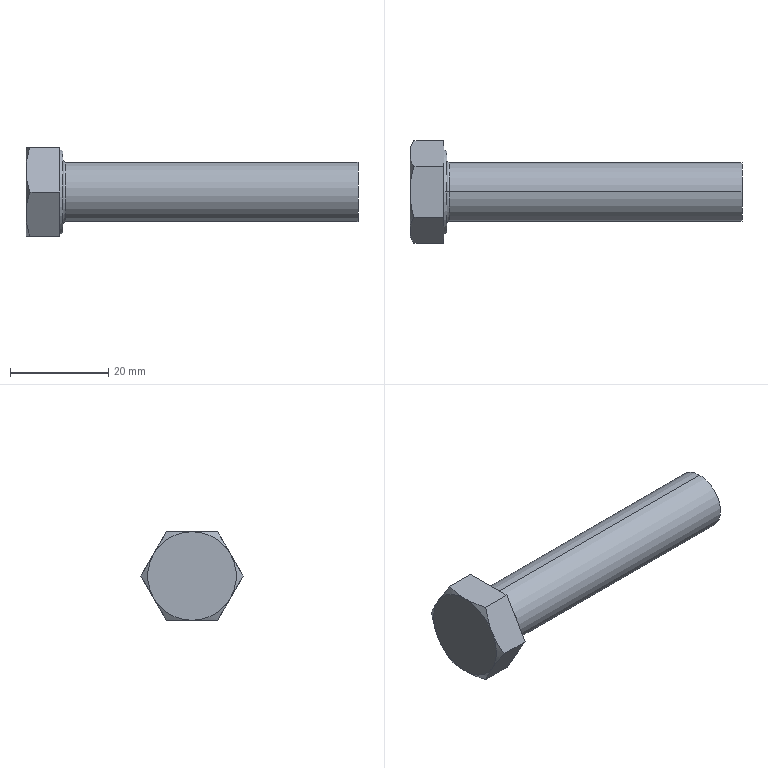Part | SolidWorks | features RevCut 3, Extrusion 1, Fillet 1, LPattern 1, Revolution 1 | 1 solid | 22 faces | box 67.5 x 20.785 x 18 mm | volume 8854 mm3 | plane 10 | cone 8 | torus 2 | cylinder 2 | commonest cylinder face diameters 12 x2
STEP:
#1=CARTESIAN_POINT('',(8.1,0.,6.));
#2=VERTEX_POINT('',#1);
#3=CARTESIAN_POINT('',(8.1,0.,-6.));
#4=VERTEX_POINT('',#3);
#5=CARTESIAN_POINT('',(8.1,0.,0.));
#6=DIRECTION('',(1.,0.,0.));
#7=DIRECTION('',(0.,0.,-1.));
#8=AXIS2_PLACEMENT_3D('',#5,#6,#7);
#9=CIRCLE('',#8,6.);
#10=EDGE_CURVE('',#2,#4,#9,.T.);
#11=ORIENTED_EDGE('',*,*,#10,.F.);
#12=CARTESIAN_POINT('',(7.5,0.,6.6));
#13=VERTEX_POINT('',#12);
#14=CARTESIAN_POINT('',(8.1,0.,6.6));
#15=DIRECTION('',(0.,1.,0.));
#16=DIRECTION('',(0.,0.,1.));
#17=AXIS2_PLACEMENT_3D('',#14,#15,#16);
#18=CIRCLE('',#17,0.6);
#19=EDGE_CURVE('',#2,#13,#18,.T.);
#20=ORIENTED_EDGE('',*,*,#19,.T.);
#21=CARTESIAN_POINT('',(7.5,0.,-6.6));
#22=VERTEX_POINT('',#21);
#23=CARTESIAN_POINT('',(7.5,0.,0.));
#24=DIRECTION('',(-1.,0.,0.));
#25=DIRECTION('',(0.,0.,-1.));
#26=AXIS2_PLACEMENT_3D('',#23,#24,#25);
#27=CIRCLE('',#26,6.6);
#28=EDGE_CURVE('',#22,#13,#27,.T.);
#29=ORIENTED_EDGE('',*,*,#28,.F.);
#30=CARTESIAN_POINT('',(8.1,0.,-6.6));
#31=DIRECTION('',(0.,-1.,0.));
#32=DIRECTION('',(0.,0.,-1.));
#33=AXIS2_PLACEMENT_3D('',#30,#31,#32);
#34=CIRCLE('',#33,0.6);
#35=EDGE_CURVE('',#4,#22,#34,.T.);
#36=ORIENTED_EDGE('',*,*,#35,.F.);
#37=EDGE_LOOP('',(#11,#20,#29,#36));
#38=FACE_OUTER_BOUND('',#37,.T.);
#39=CARTESIAN_POINT('',(8.1,0.,0.));
#40=DIRECTION('',(1.,0.,0.));
#41=DIRECTION('',(0.,0.,-1.));
#42=AXIS2_PLACEMENT_3D('',#39,#40,#41);
#43=TOROIDAL_SURFACE('',#42,6.6,0.6);
#44=ADVANCED_FACE('',(#38),#43,.F.);
#45=CARTESIAN_POINT('',(67.5,0.,6.));
#46=VERTEX_POINT('',#45);
#47=CARTESIAN_POINT('',(67.5,0.,-6.));
#48=VERTEX_POINT('',#47);
#49=CARTESIAN_POINT('',(67.5,0.,0.));
#50=DIRECTION('',(-1.,0.,0.));
#51=DIRECTION('',(0.,0.,1.));
#52=AXIS2_PLACEMENT_3D('',#49,#50,#51);
#53=CIRCLE('',#52,6.);
#54=EDGE_CURVE('',#46,#48,#53,.T.);
#55=ORIENTED_EDGE('',*,*,#54,.T.);
#56=CARTESIAN_POINT('',(0.,0.,-6.));
#57=DIRECTION('',(-1.,0.,0.));
#58=VECTOR('',#57,1000.);
#59=LINE('',#56,#58);
#60=EDGE_CURVE('',#48,#4,#59,.T.);
#61=ORIENTED_EDGE('',*,*,#60,.T.);
#62=CARTESIAN_POINT('',(8.1,0.,0.));
#63=DIRECTION('',(1.,0.,0.));
#64=DIRECTION('',(0.,0.,-1.));
#65=AXIS2_PLACEMENT_3D('',#62,#63,#64);
#66=CIRCLE('',#65,6.);
#67=EDGE_CURVE('',#4,#2,#66,.T.);
#68=ORIENTED_EDGE('',*,*,#67,.T.);
#69=CARTESIAN_POINT('',(0.,0.,6.));
#70=DIRECTION('',(-1.,0.,0.));
#71=VECTOR('',#70,1000.);
#72=LINE('',#69,#71);
#73=EDGE_CURVE('',#46,#2,#72,.T.);
#74=ORIENTED_EDGE('',*,*,#73,.F.);
#75=EDGE_LOOP('',(#55,#61,#68,#74));
#76=FACE_OUTER_BOUND('',#75,.T.);
#77=CARTESIAN_POINT('',(0.,0.,0.));
#78=DIRECTION('',(-1.,0.,0.));
#79=DIRECTION('',(0.,0.,1.));
#80=AXIS2_PLACEMENT_3D('',#77,#78,#79);
#81=CYLINDRICAL_SURFACE('',#80,6.);
#82=ADVANCED_FACE('',(#76),#81,.T.);
#83=CARTESIAN_POINT('',(7.5,0.,8.315));
#84=VERTEX_POINT('',#83);
#85=CARTESIAN_POINT('',(7.5,0.,-8.315));
#86=VERTEX_POINT('',#85);
#87=CARTESIAN_POINT('',(7.5,0.,0.));
#88=DIRECTION('',(-1.,0.,0.));
#89=DIRECTION('',(0.,0.,1.));
#90=AXIS2_PLACEMENT_3D('',#87,#88,#89);
#91=CIRCLE('',#90,8.315);
#92=EDGE_CURVE('',#84,#86,#91,.T.);
#93=ORIENTED_EDGE('',*,*,#92,.T.);
#94=CARTESIAN_POINT('',(6.9,0.,-8.661));
#95=VERTEX_POINT('',#94);
#96=CARTESIAN_POINT('',(6.9,0.,-8.661));
#97=DIRECTION('',(-0.866,0.,-0.5));
#98=VECTOR('',#97,1000.);
#99=LINE('',#96,#98);
#100=EDGE_CURVE('',#86,#95,#99,.T.);
#101=ORIENTED_EDGE('',*,*,#100,.T.);
#102=CARTESIAN_POINT('',(6.9,0.,8.661));
#103=VERTEX_POINT('',#102);
#104=CARTESIAN_POINT('',(6.9,0.,0.));
#105=DIRECTION('',(-1.,0.,0.));
#106=DIRECTION('',(0.,0.,1.));
#107=AXIS2_PLACEMENT_3D('',#104,#105,#106);
#108=CIRCLE('',#107,8.661);
#109=EDGE_CURVE('',#103,#95,#108,.T.);
#110=ORIENTED_EDGE('',*,*,#109,.F.);
#111=CARTESIAN_POINT('',(6.9,0.,8.661));
#112=DIRECTION('',(-0.866,0.,0.5));
#113=VECTOR('',#112,1000.);
#114=LINE('',#111,#113);
#115=EDGE_CURVE('',#84,#103,#114,.T.);
#116=ORIENTED_EDGE('',*,*,#115,.F.);
#117=EDGE_LOOP('',(#93,#101,#110,#116));
#118=FACE_OUTER_BOUND('',#117,.T.);
#119=CARTESIAN_POINT('',(6.9,0.,0.));
#120=DIRECTION('',(-1.,0.,0.));
#121=DIRECTION('',(0.,0.,1.));
#122=AXIS2_PLACEMENT_3D('',#119,#120,#121);
#123=CONICAL_SURFACE('',#122,8.661,0.5236);
#124=ADVANCED_FACE('',(#118),#123,.T.);
#125=CARTESIAN_POINT('',(6.9,5.196,-9.));
#126=VERTEX_POINT('',#125);
#127=CARTESIAN_POINT('',(6.9,10.392,0.));
#128=VERTEX_POINT('',#127);
#129=CARTESIAN_POINT('',(6.9,5.196,-9.));
#130=DIRECTION('',(0.,0.5,0.866));
#131=VECTOR('',#130,1000.);
#132=LINE('',#129,#131);
#133=EDGE_CURVE('',#126,#128,#132,.T.);
#134=ORIENTED_EDGE('',*,*,#133,.F.);
#135=CARTESIAN_POINT('',(0.8038,5.196,-9.));
#136=VERTEX_POINT('',#135);
#137=CARTESIAN_POINT('',(7.5,5.196,-9.));
#138=DIRECTION('',(-1.,0.,0.));
#139=VECTOR('',#138,1000.);
#140=LINE('',#137,#139);
#141=EDGE_CURVE('',#126,#136,#140,.T.);
#142=ORIENTED_EDGE('',*,*,#141,.T.);
#143=CARTESIAN_POINT('',(0.,7.794,-4.5));
#144=VERTEX_POINT('',#143);
#145=CARTESIAN_POINT('',(0.,7.794,-4.5));
#146=CARTESIAN_POINT('',(0.,7.574,-4.882));
#147=CARTESIAN_POINT('',(0.019,7.352,-5.266));
#148=CARTESIAN_POINT('',(0.09253,6.914,-6.024));
#149=CARTESIAN_POINT('',(0.147,6.697,-6.401));
#150=CARTESIAN_POINT('',(0.357,6.048,-7.525));
#151=CARTESIAN_POINT('',(0.5591,5.62,-8.266));
#152=CARTESIAN_POINT('',(0.8038,5.196,-9.));
#153=B_SPLINE_CURVE_WITH_KNOTS('',3,(#145,#146,#147,#148,#149,#150,#151,#152),.UNSPECIFIED.,.F.,.F.,(4,2,2,4),(0.005258,0.006567,0.007877,0.0105),.UNSPECIFIED.);
#154=EDGE_CURVE('',#144,#136,#153,.T.);
#155=ORIENTED_EDGE('',*,*,#154,.F.);
#156=CARTESIAN_POINT('',(0.8038,10.392,0.));
#157=VERTEX_POINT('',#156);
#158=CARTESIAN_POINT('',(0.8038,10.392,0.));
#159=CARTESIAN_POINT('',(0.5585,9.967,-0.7361));
#160=CARTESIAN_POINT('',(0.3563,9.539,-1.478));
#161=CARTESIAN_POINT('',(0.07661,8.674,-2.976));
#162=CARTESIAN_POINT('',(0.,8.237,-3.733));
#163=CARTESIAN_POINT('',(0.,7.794,-4.5));
#164=B_SPLINE_CURVE_WITH_KNOTS('',3,(#158,#159,#160,#161,#162,#163),.UNSPECIFIED.,.F.,.F.,(4,2,4),(0.000000238,0.002629,0.005258),.UNSPECIFIED.);
#165=EDGE_CURVE('',#157,#144,#164,.T.);
#166=ORIENTED_EDGE('',*,*,#165,.F.);
#167=CARTESIAN_POINT('',(7.5,10.392,0.));
#168=DIRECTION('',(-1.,0.,0.));
#169=VECTOR('',#168,1000.);
#170=LINE('',#167,#169);
#171=EDGE_CURVE('',#128,#157,#170,.T.);
#172=ORIENTED_EDGE('',*,*,#171,.F.);
#173=EDGE_LOOP('',(#134,#142,#155,#166,#172));
#174=FACE_OUTER_BOUND('',#173,.T.);
#175=CARTESIAN_POINT('',(7.5,5.196,-9.));
#176=DIRECTION('',(0.,-0.866,0.5));
#177=DIRECTION('',(0.,-0.5,-0.866));
#178=AXIS2_PLACEMENT_3D('',#175,#176,#177);
#179=PLANE('',#178);
#180=ADVANCED_FACE('',(#174),#179,.F.);
#181=CARTESIAN_POINT('',(6.9,5.196,9.));
#182=VERTEX_POINT('',#181);
#183=CARTESIAN_POINT('',(6.9,10.392,0.));
#184=DIRECTION('',(0.,-0.5,0.866));
#185=VECTOR('',#184,1000.);
#186=LINE('',#183,#185);
#187=EDGE_CURVE('',#128,#182,#186,.T.);
#188=ORIENTED_EDGE('',*,*,#187,.F.);
#189=ORIENTED_EDGE('',*,*,#171,.T.);
#190=CARTESIAN_POINT('',(0.,7.794,4.5));
#191=VERTEX_POINT('',#190);
#192=CARTESIAN_POINT('',(0.,7.794,4.5));
#193=CARTESIAN_POINT('',(0.,8.015,4.118));
#194=CARTESIAN_POINT('',(0.019,8.236,3.734));
#195=CARTESIAN_POINT('',(0.09253,8.674,2.976));
#196=CARTESIAN_POINT('',(0.147,8.892,2.599));
#197=CARTESIAN_POINT('',(0.357,9.541,1.475));
#198=CARTESIAN_POINT('',(0.5591,9.968,0.7343));
#199=CARTESIAN_POINT('',(0.8038,10.392,0.));
#200=B_SPLINE_CURVE_WITH_KNOTS('',3,(#192,#193,#194,#195,#196,#197,#198,#199),.UNSPECIFIED.,.F.,.F.,(4,2,2,4),(0.005258,0.006567,0.007877,0.0105),.UNSPECIFIED.);
#201=EDGE_CURVE('',#191,#157,#200,.T.);
#202=ORIENTED_EDGE('',*,*,#201,.F.);
#203=CARTESIAN_POINT('',(0.8038,5.196,9.));
#204=VERTEX_POINT('',#203);
#205=CARTESIAN_POINT('',(0.8038,5.196,9.));
#206=CARTESIAN_POINT('',(0.5585,5.621,8.264));
#207=CARTESIAN_POINT('',(0.3563,6.049,7.522));
#208=CARTESIAN_POINT('',(0.07661,6.914,6.024));
#209=CARTESIAN_POINT('',(0.,7.352,5.267));
#210=CARTESIAN_POINT('',(0.,7.794,4.5));
#211=B_SPLINE_CURVE_WITH_KNOTS('',3,(#205,#206,#207,#208,#209,#210),.UNSPECIFIED.,.F.,.F.,(4,2,4),(0.000000238,0.002629,0.005258),.UNSPECIFIED.);
#212=EDGE_CURVE('',#204,#191,#211,.T.);
#213=ORIENTED_EDGE('',*,*,#212,.F.);
#214=CARTESIAN_POINT('',(7.5,5.196,9.));
#215=DIRECTION('',(-1.,0.,0.));
#216=VECTOR('',#215,1000.);
#217=LINE('',#214,#216);
#218=EDGE_CURVE('',#182,#204,#217,.T.);
#219=ORIENTED_EDGE('',*,*,#218,.F.);
#220=EDGE_LOOP('',(#188,#189,#202,#213,#219));
#221=FACE_OUTER_BOUND('',#220,.T.);
#222=CARTESIAN_POINT('',(7.5,10.392,0.));
#223=DIRECTION('',(0.,-0.866,-0.5));
#224=DIRECTION('',(0.,0.5,-0.866));
#225=AXIS2_PLACEMENT_3D('',#222,#223,#224);
#226=PLANE('',#225);
#227=ADVANCED_FACE('',(#221),#226,.F.);
#228=CARTESIAN_POINT('',(6.9,-5.196,9.));
#229=VERTEX_POINT('',#228);
#230=CARTESIAN_POINT('',(6.9,5.196,9.));
#231=DIRECTION('',(0.,-1.,0.));
#232=VECTOR('',#231,1000.);
#233=LINE('',#230,#232);
#234=EDGE_CURVE('',#182,#229,#233,.T.);
#235=ORIENTED_EDGE('',*,*,#234,.F.);
#236=ORIENTED_EDGE('',*,*,#218,.T.);
#237=CARTESIAN_POINT('',(0.,0.,9.));
#238=VERTEX_POINT('',#237);
#239=CARTESIAN_POINT('',(0.,0.,9.));
#240=CARTESIAN_POINT('',(0.,0.4401,9.));
#241=CARTESIAN_POINT('',(0.01885,0.8832,9.));
#242=CARTESIAN_POINT('',(0.09319,1.767,9.));
#243=CARTESIAN_POINT('',(0.1482,2.204,9.));
#244=CARTESIAN_POINT('',(0.3593,3.505,9.));
#245=CARTESIAN_POINT('',(0.5612,4.356,9.));
#246=CARTESIAN_POINT('',(0.8038,5.196,9.));
#247=B_SPLINE_CURVE_WITH_KNOTS('',3,(#239,#240,#241,#242,#243,#244,#245,#246),.UNSPECIFIED.,.F.,.F.,(4,2,2,4),(0.01498,0.0163,0.01761,0.02025),.UNSPECIFIED.);
#248=EDGE_CURVE('',#238,#204,#247,.T.);
#249=ORIENTED_EDGE('',*,*,#248,.F.);
#250=CARTESIAN_POINT('',(0.8038,-5.196,9.));
#251=VERTEX_POINT('',#250);
#252=CARTESIAN_POINT('',(0.8038,-5.196,9.));
#253=CARTESIAN_POINT('',(0.5595,-4.35,9.));
#254=CARTESIAN_POINT('',(0.3552,-3.485,9.));
#255=CARTESIAN_POINT('',(0.07569,-1.752,9.));
#256=CARTESIAN_POINT('',(0.,-0.8794,9.));
#257=CARTESIAN_POINT('',(0.,0.,9.));
#258=B_SPLINE_CURVE_WITH_KNOTS('',3,(#252,#253,#254,#255,#256,#257),.UNSPECIFIED.,.F.,.F.,(4,2,4),(0.00972,0.01235,0.01498),.UNSPECIFIED.);
#259=EDGE_CURVE('',#251,#238,#258,.T.);
#260=ORIENTED_EDGE('',*,*,#259,.F.);
#261=CARTESIAN_POINT('',(7.5,-5.196,9.));
#262=DIRECTION('',(-1.,0.,0.));
#263=VECTOR('',#262,1000.);
#264=LINE('',#261,#263);
#265=EDGE_CURVE('',#229,#251,#264,.T.);
#266=ORIENTED_EDGE('',*,*,#265,.F.);
#267=EDGE_LOOP('',(#235,#236,#249,#260,#266));
#268=FACE_OUTER_BOUND('',#267,.T.);
#269=CARTESIAN_POINT('',(7.5,5.196,9.));
#270=DIRECTION('',(0.,0.,-1.));
#271=DIRECTION('',(-1.,0.,0.));
#272=AXIS2_PLACEMENT_3D('',#269,#270,#271);
#273=PLANE('',#272);
#274=ADVANCED_FACE('',(#268),#273,.F.);
#275=CARTESIAN_POINT('',(6.9,-10.392,0.));
#276=VERTEX_POINT('',#275);
#277=CARTESIAN_POINT('',(6.9,-10.392,0.));
#278=DIRECTION('',(0.,-0.5,-0.866));
#279=VECTOR('',#278,1000.);
#280=LINE('',#277,#279);
#281=EDGE_CURVE('',#229,#276,#280,.T.);
#282=ORIENTED_EDGE('',*,*,#281,.F.);
#283=ORIENTED_EDGE('',*,*,#265,.T.);
#284=CARTESIAN_POINT('',(0.,-7.794,4.5));
#285=VERTEX_POINT('',#284);
#286=CARTESIAN_POINT('',(0.,-7.794,4.5));
#287=CARTESIAN_POINT('',(0.,-7.574,4.882));
#288=CARTESIAN_POINT('',(0.019,-7.352,5.266));
#289=CARTESIAN_POINT('',(0.09253,-6.914,6.024));
#290=CARTESIAN_POINT('',(0.147,-6.697,6.401));
#291=CARTESIAN_POINT('',(0.357,-6.048,7.525));
#292=CARTESIAN_POINT('',(0.5591,-5.62,8.266));
#293=CARTESIAN_POINT('',(0.8038,-5.196,9.));
#294=B_SPLINE_CURVE_WITH_KNOTS('',3,(#286,#287,#288,#289,#290,#291,#292,#293),.UNSPECIFIED.,.F.,.F.,(4,2,2,4),(0.005258,0.006567,0.007877,0.0105),.UNSPECIFIED.);
#295=EDGE_CURVE('',#285,#251,#294,.T.);
#296=ORIENTED_EDGE('',*,*,#295,.F.);
#297=CARTESIAN_POINT('',(0.8038,-10.392,0.));
#298=VERTEX_POINT('',#297);
#299=CARTESIAN_POINT('',(0.8038,-10.392,0.));
#300=CARTESIAN_POINT('',(0.5585,-9.967,0.7361));
#301=CARTESIAN_POINT('',(0.3563,-9.539,1.478));
#302=CARTESIAN_POINT('',(0.07661,-8.674,2.976));
#303=CARTESIAN_POINT('',(0.,-8.237,3.733));
#304=CARTESIAN_POINT('',(0.,-7.794,4.5));
#305=B_SPLINE_CURVE_WITH_KNOTS('',3,(#299,#300,#301,#302,#303,#304),.UNSPECIFIED.,.F.,.F.,(4,2,4),(0.000000238,0.002629,0.005258),.UNSPECIFIED.);
#306=EDGE_CURVE('',#298,#285,#305,.T.);
#307=ORIENTED_EDGE('',*,*,#306,.F.);
#308=CARTESIAN_POINT('',(7.5,-10.392,0.));
#309=DIRECTION('',(-1.,0.,0.));
#310=VECTOR('',#309,1000.);
#311=LINE('',#308,#310);
#312=EDGE_CURVE('',#276,#298,#311,.T.);
#313=ORIENTED_EDGE('',*,*,#312,.F.);
#314=EDGE_LOOP('',(#282,#283,#296,#307,#313));
#315=FACE_OUTER_BOUND('',#314,.T.);
#316=CARTESIAN_POINT('',(7.5,-10.392,0.));
#317=DIRECTION('',(0.,0.866,-0.5));
#318=DIRECTION('',(0.,0.5,0.866));
#319=AXIS2_PLACEMENT_3D('',#316,#317,#318);
#320=PLANE('',#319);
#321=ADVANCED_FACE('',(#315),#320,.F.);
#322=CARTESIAN_POINT('',(6.9,-5.196,-9.));
#323=VERTEX_POINT('',#322);
#324=CARTESIAN_POINT('',(6.9,-5.196,-9.));
#325=DIRECTION('',(0.,0.5,-0.866));
#326=VECTOR('',#325,1000.);
#327=LINE('',#324,#326);
#328=EDGE_CURVE('',#276,#323,#327,.T.);
#329=ORIENTED_EDGE('',*,*,#328,.F.);
#330=ORIENTED_EDGE('',*,*,#312,.T.);
#331=CARTESIAN_POINT('',(0.,-7.794,-4.5));
#332=VERTEX_POINT('',#331);
#333=CARTESIAN_POINT('',(0.,-7.794,-4.5));
#334=CARTESIAN_POINT('',(0.,-8.015,-4.118));
#335=CARTESIAN_POINT('',(0.019,-8.236,-3.734));
#336=CARTESIAN_POINT('',(0.09253,-8.674,-2.976));
#337=CARTESIAN_POINT('',(0.147,-8.892,-2.599));
#338=CARTESIAN_POINT('',(0.357,-9.541,-1.475));
#339=CARTESIAN_POINT('',(0.5591,-9.968,-0.7343));
#340=CARTESIAN_POINT('',(0.8038,-10.392,0.));
#341=B_SPLINE_CURVE_WITH_KNOTS('',3,(#333,#334,#335,#336,#337,#338,#339,#340),.UNSPECIFIED.,.F.,.F.,(4,2,2,4),(0.005258,0.006567,0.007877,0.0105),.UNSPECIFIED.);
#342=EDGE_CURVE('',#332,#298,#341,.T.);
#343=ORIENTED_EDGE('',*,*,#342,.F.);
#344=CARTESIAN_POINT('',(0.8038,-5.196,-9.));
#345=VERTEX_POINT('',#344);
#346=CARTESIAN_POINT('',(0.8038,-5.196,-9.));
#347=CARTESIAN_POINT('',(0.5585,-5.621,-8.264));
#348=CARTESIAN_POINT('',(0.3563,-6.049,-7.522));
#349=CARTESIAN_POINT('',(0.07661,-6.914,-6.024));
#350=CARTESIAN_POINT('',(0.,-7.352,-5.267));
#351=CARTESIAN_POINT('',(0.,-7.794,-4.5));
#352=B_SPLINE_CURVE_WITH_KNOTS('',3,(#346,#347,#348,#349,#350,#351),.UNSPECIFIED.,.F.,.F.,(4,2,4),(0.000000238,0.002629,0.005258),.UNSPECIFIED.);
#353=EDGE_CURVE('',#345,#332,#352,.T.);
#354=ORIENTED_EDGE('',*,*,#353,.F.);
#355=CARTESIAN_POINT('',(7.5,-5.196,-9.));
#356=DIRECTION('',(-1.,0.,0.));
#357=VECTOR('',#356,1000.);
#358=LINE('',#355,#357);
#359=EDGE_CURVE('',#323,#345,#358,.T.);
#360=ORIENTED_EDGE('',*,*,#359,.F.);
#361=EDGE_LOOP('',(#329,#330,#343,#354,#360));
#362=FACE_OUTER_BOUND('',#361,.T.);
#363=CARTESIAN_POINT('',(7.5,-5.196,-9.));
#364=DIRECTION('',(0.,0.866,0.5));
#365=DIRECTION('',(0.,-0.5,0.866));
#366=AXIS2_PLACEMENT_3D('',#363,#364,#365);
#367=PLANE('',#366);
#368=ADVANCED_FACE('',(#362),#367,.F.);
#369=CARTESIAN_POINT('',(6.9,5.196,-9.));
#370=DIRECTION('',(0.,1.,0.));
#371=VECTOR('',#370,1000.);
#372=LINE('',#369,#371);
#373=EDGE_CURVE('',#323,#126,#372,.T.);
#374=ORIENTED_EDGE('',*,*,#373,.F.);
#375=ORIENTED_EDGE('',*,*,#359,.T.);
#376=CARTESIAN_POINT('',(0.,0.,-9.));
#377=VERTEX_POINT('',#376);
#378=CARTESIAN_POINT('',(0.,0.,-9.));
#379=CARTESIAN_POINT('',(0.,-0.8794,-9.));
#380=CARTESIAN_POINT('',(0.07569,-1.752,-9.));
#381=CARTESIAN_POINT('',(0.3552,-3.485,-9.));
#382=CARTESIAN_POINT('',(0.5595,-4.35,-9.));
#383=CARTESIAN_POINT('',(0.8038,-5.196,-9.));
#384=B_SPLINE_CURVE_WITH_KNOTS('',3,(#378,#379,#380,#381,#382,#383),.UNSPECIFIED.,.F.,.F.,(4,2,4),(0.03045,0.03308,0.03571),.UNSPECIFIED.);
#385=EDGE_CURVE('',#377,#345,#384,.T.);
#386=ORIENTED_EDGE('',*,*,#385,.F.);
#387=CARTESIAN_POINT('',(0.8038,5.196,-9.));
#388=CARTESIAN_POINT('',(0.5612,4.356,-9.));
#389=CARTESIAN_POINT('',(0.3593,3.505,-9.));
#390=CARTESIAN_POINT('',(0.1482,2.204,-9.));
#391=CARTESIAN_POINT('',(0.09319,1.767,-9.));
#392=CARTESIAN_POINT('',(0.01885,0.8832,-9.));
#393=CARTESIAN_POINT('',(0.,0.4401,-9.));
#394=CARTESIAN_POINT('',(0.,0.,-9.));
#395=B_SPLINE_CURVE_WITH_KNOTS('',3,(#387,#388,#389,#390,#391,#392,#393,#394),.UNSPECIFIED.,.F.,.F.,(4,2,2,4),(0.02519,0.02782,0.02914,0.03045),.UNSPECIFIED.);
#396=EDGE_CURVE('',#136,#377,#395,.T.);
#397=ORIENTED_EDGE('',*,*,#396,.F.);
#398=ORIENTED_EDGE('',*,*,#141,.F.);
#399=EDGE_LOOP('',(#374,#375,#386,#397,#398));
#400=FACE_OUTER_BOUND('',#399,.T.);
#401=CARTESIAN_POINT('',(7.5,5.196,-9.));
#402=DIRECTION('',(0.,0.,1.));
#403=DIRECTION('',(0.,-1.,0.));
#404=AXIS2_PLACEMENT_3D('',#401,#402,#403);
#405=PLANE('',#404);
#406=ADVANCED_FACE('',(#400),#405,.F.);
#407=ORIENTED_EDGE('',*,*,#353,.T.);
#408=CARTESIAN_POINT('',(0.,0.,0.));
#409=DIRECTION('',(1.,0.,0.));
#410=DIRECTION('',(0.,0.,-1.));
#411=AXIS2_PLACEMENT_3D('',#408,#409,#410);
#412=CIRCLE('',#411,9.);
#413=EDGE_CURVE('',#332,#377,#412,.T.);
#414=ORIENTED_EDGE('',*,*,#413,.T.);
#415=ORIENTED_EDGE('',*,*,#385,.T.);
#416=EDGE_LOOP('',(#407,#414,#415));
#417=FACE_OUTER_BOUND('',#416,.T.);
#418=CARTESIAN_POINT('',(0.,0.,0.));
#419=DIRECTION('',(1.,0.,0.));
#420=DIRECTION('',(0.,0.,-1.));
#421=AXIS2_PLACEMENT_3D('',#418,#419,#420);
#422=CONICAL_SURFACE('',#421,9.,1.047);
#423=ADVANCED_FACE('',(#417),#422,.T.);
#424=ORIENTED_EDGE('',*,*,#306,.T.);
#425=CARTESIAN_POINT('',(0.,0.,0.));
#426=DIRECTION('',(1.,0.,0.));
#427=DIRECTION('',(0.,0.,-1.));
#428=AXIS2_PLACEMENT_3D('',#425,#426,#427);
#429=CIRCLE('',#428,9.);
#430=EDGE_CURVE('',#285,#332,#429,.T.);
#431=ORIENTED_EDGE('',*,*,#430,.T.);
#432=ORIENTED_EDGE('',*,*,#342,.T.);
#433=EDGE_LOOP('',(#424,#431,#432));
#434=FACE_OUTER_BOUND('',#433,.T.);
#435=CARTESIAN_POINT('',(0.,0.,0.));
#436=DIRECTION('',(1.,0.,0.));
#437=DIRECTION('',(0.,0.,-1.));
#438=AXIS2_PLACEMENT_3D('',#435,#436,#437);
#439=CONICAL_SURFACE('',#438,9.,1.047);
#440=ADVANCED_FACE('',(#434),#439,.T.);
#441=ORIENTED_EDGE('',*,*,#259,.T.);
#442=CARTESIAN_POINT('',(0.,0.,0.));
#443=DIRECTION('',(1.,0.,0.));
#444=DIRECTION('',(0.,0.,-1.));
#445=AXIS2_PLACEMENT_3D('',#442,#443,#444);
#446=CIRCLE('',#445,9.);
#447=EDGE_CURVE('',#238,#285,#446,.T.);
#448=ORIENTED_EDGE('',*,*,#447,.T.);
#449=ORIENTED_EDGE('',*,*,#295,.T.);
#450=EDGE_LOOP('',(#441,#448,#449));
#451=FACE_OUTER_BOUND('',#450,.T.);
#452=CARTESIAN_POINT('',(0.,0.,0.));
#453=DIRECTION('',(1.,0.,0.));
#454=DIRECTION('',(0.,0.,-1.));
#455=AXIS2_PLACEMENT_3D('',#452,#453,#454);
#456=CONICAL_SURFACE('',#455,9.,1.047);
#457=ADVANCED_FACE('',(#451),#456,.T.);
#458=ORIENTED_EDGE('',*,*,#248,.T.);
#459=ORIENTED_EDGE('',*,*,#212,.T.);
#460=CARTESIAN_POINT('',(0.,0.,0.));
#461=DIRECTION('',(-1.,0.,0.));
#462=DIRECTION('',(0.,0.,1.));
#463=AXIS2_PLACEMENT_3D('',#460,#461,#462);
#464=CIRCLE('',#463,9.);
#465=EDGE_CURVE('',#238,#191,#464,.T.);
#466=ORIENTED_EDGE('',*,*,#465,.F.);
#467=EDGE_LOOP('',(#458,#459,#466));
#468=FACE_OUTER_BOUND('',#467,.T.);
#469=CARTESIAN_POINT('',(0.,0.,0.));
#470=DIRECTION('',(1.,0.,0.));
#471=DIRECTION('',(0.,0.,-1.));
#472=AXIS2_PLACEMENT_3D('',#469,#470,#471);
#473=CONICAL_SURFACE('',#472,9.,1.047);
#474=ADVANCED_FACE('',(#468),#473,.T.);
#475=ORIENTED_EDGE('',*,*,#201,.T.);
#476=ORIENTED_EDGE('',*,*,#165,.T.);
#477=CARTESIAN_POINT('',(0.,0.,0.));
#478=DIRECTION('',(1.,0.,0.));
#479=DIRECTION('',(0.,0.,-1.));
#480=AXIS2_PLACEMENT_3D('',#477,#478,#479);
#481=CIRCLE('',#480,9.);
#482=EDGE_CURVE('',#144,#191,#481,.T.);
#483=ORIENTED_EDGE('',*,*,#482,.T.);
#484=EDGE_LOOP('',(#475,#476,#483));
#485=FACE_OUTER_BOUND('',#484,.T.);
#486=CARTESIAN_POINT('',(0.,0.,0.));
#487=DIRECTION('',(1.,0.,0.));
#488=DIRECTION('',(0.,0.,-1.));
#489=AXIS2_PLACEMENT_3D('',#486,#487,#488);
#490=CONICAL_SURFACE('',#489,9.,1.047);
#491=ADVANCED_FACE('',(#485),#490,.T.);
#492=ORIENTED_EDGE('',*,*,#154,.T.);
#493=ORIENTED_EDGE('',*,*,#396,.T.);
#494=CARTESIAN_POINT('',(0.,0.,0.));
#495=DIRECTION('',(1.,0.,0.));
#496=DIRECTION('',(0.,0.,-1.));
#497=AXIS2_PLACEMENT_3D('',#494,#495,#496);
#498=CIRCLE('',#497,9.);
#499=EDGE_CURVE('',#377,#144,#498,.T.);
#500=ORIENTED_EDGE('',*,*,#499,.T.);
#501=EDGE_LOOP('',(#492,#493,#500));
#502=FACE_OUTER_BOUND('',#501,.T.);
#503=CARTESIAN_POINT('',(0.,0.,0.));
#504=DIRECTION('',(1.,0.,0.));
#505=DIRECTION('',(0.,0.,-1.));
#506=AXIS2_PLACEMENT_3D('',#503,#504,#505);
#507=CONICAL_SURFACE('',#506,9.,1.047);
#508=ADVANCED_FACE('',(#502),#507,.T.);
#509=ORIENTED_EDGE('',*,*,#499,.F.);
#510=ORIENTED_EDGE('',*,*,#413,.F.);
#511=ORIENTED_EDGE('',*,*,#430,.F.);
#512=ORIENTED_EDGE('',*,*,#447,.F.);
#513=ORIENTED_EDGE('',*,*,#465,.T.);
#514=ORIENTED_EDGE('',*,*,#482,.F.);
#515=EDGE_LOOP('',(#509,#510,#511,#512,#513,#514));
#516=FACE_OUTER_BOUND('',#515,.T.);
#517=CARTESIAN_POINT('',(0.,10.392,0.));
#518=DIRECTION('',(1.,0.,0.));
#519=DIRECTION('',(0.,0.,-1.));
#520=AXIS2_PLACEMENT_3D('',#517,#518,#519);
#521=PLANE('',#520);
#522=ADVANCED_FACE('',(#516),#521,.F.);
#523=ORIENTED_EDGE('',*,*,#109,.T.);
#524=CARTESIAN_POINT('',(6.9,0.,0.));
#525=DIRECTION('',(-1.,0.,0.));
#526=DIRECTION('',(0.,0.,1.));
#527=AXIS2_PLACEMENT_3D('',#524,#525,#526);
#528=CIRCLE('',#527,8.661);
#529=EDGE_CURVE('',#95,#103,#528,.T.);
#530=ORIENTED_EDGE('',*,*,#529,.T.);
#531=EDGE_LOOP('',(#523,#530));
#532=FACE_BOUND('',#531,.T.);
#533=ORIENTED_EDGE('',*,*,#133,.T.);
#534=ORIENTED_EDGE('',*,*,#187,.T.);
#535=ORIENTED_EDGE('',*,*,#234,.T.);
#536=ORIENTED_EDGE('',*,*,#281,.T.);
#537=ORIENTED_EDGE('',*,*,#328,.T.);
#538=ORIENTED_EDGE('',*,*,#373,.T.);
#539=EDGE_LOOP('',(#533,#534,#535,#536,#537,#538));
#540=FACE_OUTER_BOUND('',#539,.T.);
#541=CARTESIAN_POINT('',(6.9,8.661,0.));
#542=DIRECTION('',(1.,0.,0.));
#543=DIRECTION('',(0.,0.,-1.));
#544=AXIS2_PLACEMENT_3D('',#541,#542,#543);
#545=PLANE('',#544);
#546=ADVANCED_FACE('',(#532,#540),#545,.T.);
#547=ORIENTED_EDGE('',*,*,#100,.F.);
#548=CARTESIAN_POINT('',(7.5,0.,0.));
#549=DIRECTION('',(-1.,0.,0.));
#550=DIRECTION('',(0.,0.,1.));
#551=AXIS2_PLACEMENT_3D('',#548,#549,#550);
#552=CIRCLE('',#551,8.315);
#553=EDGE_CURVE('',#86,#84,#552,.T.);
#554=ORIENTED_EDGE('',*,*,#553,.T.);
#555=ORIENTED_EDGE('',*,*,#115,.T.);
#556=ORIENTED_EDGE('',*,*,#529,.F.);
#557=EDGE_LOOP('',(#547,#554,#555,#556));
#558=FACE_OUTER_BOUND('',#557,.T.);
#559=CARTESIAN_POINT('',(6.9,0.,0.));
#560=DIRECTION('',(-1.,0.,0.));
#561=DIRECTION('',(0.,0.,1.));
#562=AXIS2_PLACEMENT_3D('',#559,#560,#561);
#563=CONICAL_SURFACE('',#562,8.661,0.5236);
#564=ADVANCED_FACE('',(#558),#563,.T.);
#565=ORIENTED_EDGE('',*,*,#54,.F.);
#566=CARTESIAN_POINT('',(67.5,0.,0.));
#567=DIRECTION('',(-1.,0.,0.));
#568=DIRECTION('',(0.,0.,1.));
#569=AXIS2_PLACEMENT_3D('',#566,#567,#568);
#570=CIRCLE('',#569,6.);
#571=EDGE_CURVE('',#48,#46,#570,.T.);
#572=ORIENTED_EDGE('',*,*,#571,.F.);
#573=EDGE_LOOP('',(#565,#572));
#574=FACE_OUTER_BOUND('',#573,.T.);
#575=CARTESIAN_POINT('',(67.5,0.,0.));
#576=DIRECTION('',(-1.,0.,0.));
#577=DIRECTION('',(0.,0.,1.));
#578=AXIS2_PLACEMENT_3D('',#575,#576,#577);
#579=PLANE('',#578);
#580=ADVANCED_FACE('',(#574),#579,.F.);
#581=ORIENTED_EDGE('',*,*,#60,.F.);
#582=ORIENTED_EDGE('',*,*,#571,.T.);
#583=ORIENTED_EDGE('',*,*,#73,.T.);
#584=ORIENTED_EDGE('',*,*,#10,.T.);
#585=EDGE_LOOP('',(#581,#582,#583,#584));
#586=FACE_OUTER_BOUND('',#585,.T.);
#587=CARTESIAN_POINT('',(0.,0.,0.));
#588=DIRECTION('',(-1.,0.,0.));
#589=DIRECTION('',(0.,0.,1.));
#590=AXIS2_PLACEMENT_3D('',#587,#588,#589);
#591=CYLINDRICAL_SURFACE('',#590,6.);
#592=ADVANCED_FACE('',(#586),#591,.T.);
#593=ORIENTED_EDGE('',*,*,#28,.T.);
#594=CARTESIAN_POINT('',(7.5,0.,0.));
#595=DIRECTION('',(-1.,0.,0.));
#596=DIRECTION('',(0.,0.,-1.));
#597=AXIS2_PLACEMENT_3D('',#594,#595,#596);
#598=CIRCLE('',#597,6.6);
#599=EDGE_CURVE('',#13,#22,#598,.T.);
#600=ORIENTED_EDGE('',*,*,#599,.T.);
#601=EDGE_LOOP('',(#593,#600));
#602=FACE_BOUND('',#601,.T.);
#603=ORIENTED_EDGE('',*,*,#92,.F.);
#604=ORIENTED_EDGE('',*,*,#553,.F.);
#605=EDGE_LOOP('',(#603,#604));
#606=FACE_OUTER_BOUND('',#605,.T.);
#607=CARTESIAN_POINT('',(7.5,10.392,0.));
#608=DIRECTION('',(1.,0.,0.));
#609=DIRECTION('',(0.,0.,-1.));
#610=AXIS2_PLACEMENT_3D('',#607,#608,#609);
#611=PLANE('',#610);
#612=ADVANCED_FACE('',(#602,#606),#611,.T.);
#613=ORIENTED_EDGE('',*,*,#19,.F.);
#614=ORIENTED_EDGE('',*,*,#67,.F.);
#615=ORIENTED_EDGE('',*,*,#35,.T.);
#616=ORIENTED_EDGE('',*,*,#599,.F.);
#617=EDGE_LOOP('',(#613,#614,#615,#616));
#618=FACE_OUTER_BOUND('',#617,.T.);
#619=CARTESIAN_POINT('',(8.1,0.,0.));
#620=DIRECTION('',(1.,0.,0.));
#621=DIRECTION('',(0.,0.,-1.));
#622=AXIS2_PLACEMENT_3D('',#619,#620,#621);
#623=TOROIDAL_SURFACE('',#622,6.6,0.6);
#624=ADVANCED_FACE('',(#618),#623,.F.);
#625=CLOSED_SHELL('',(#44,#82,#124,#180,#227,#274,#321,#368,#406,#423,#440,#457,#474,#491,#508,#522,#546,#564,#580,#592,#612,#624));
#626=MANIFOLD_SOLID_BREP('',#625);
#627=CARTESIAN_POINT('',(0.,0.,0.));
#628=DIRECTION('',(0.,0.,1.));
#629=DIRECTION('',(1.,0.,0.));
#630=AXIS2_PLACEMENT_3D('',#627,#628,#629);
#631=(LENGTH_UNIT()NAMED_UNIT(*)SI_UNIT(.MILLI.,.METRE.));
#632=UNCERTAINTY_MEASURE_WITH_UNIT(LENGTH_MEASURE(0.00001),#631,'','');
#633=(NAMED_UNIT(*)PLANE_ANGLE_UNIT()SI_UNIT($,.RADIAN.));
#634=(NAMED_UNIT(*)SI_UNIT($,.STERADIAN.)SOLID_ANGLE_UNIT());
#635=(GEOMETRIC_REPRESENTATION_CONTEXT(3)GLOBAL_UNCERTAINTY_ASSIGNED_CONTEXT((#632))GLOBAL_UNIT_ASSIGNED_CONTEXT((#631,#633,#634))REPRESENTATION_CONTEXT('',''));
#636=ADVANCED_BREP_SHAPE_REPRESENTATION('',(#626,#630),#635);